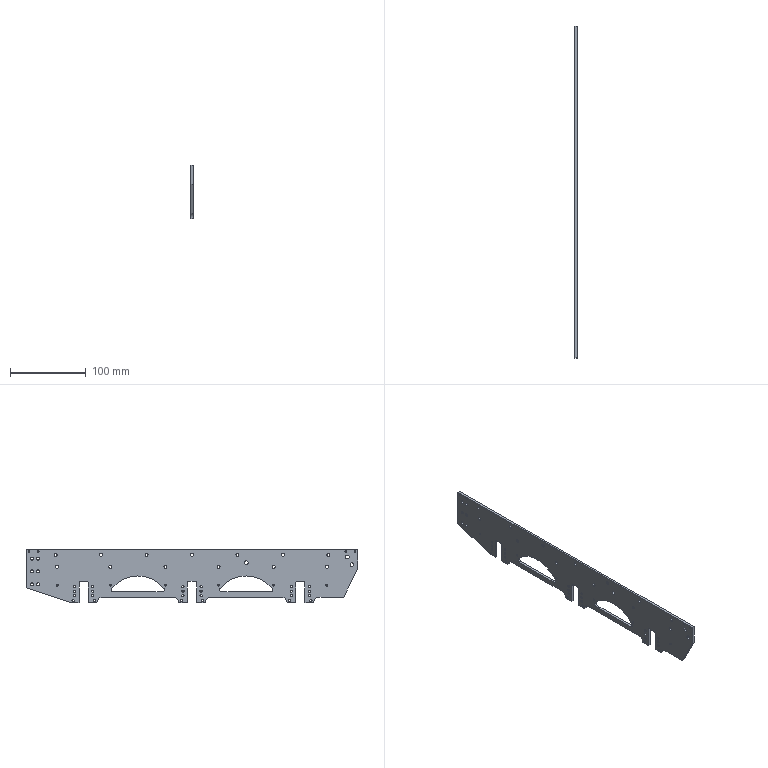Part | STEP file | 1-40.1 | 1 solid | 100 faces | box 3 x 438 x 70 mm | volume 72359 mm3 | cylinder 73 | plane 27 | commonest cylinder face diameters 4 x25 3 x24 2.5 x10 14 x5 6 x4 5 x3